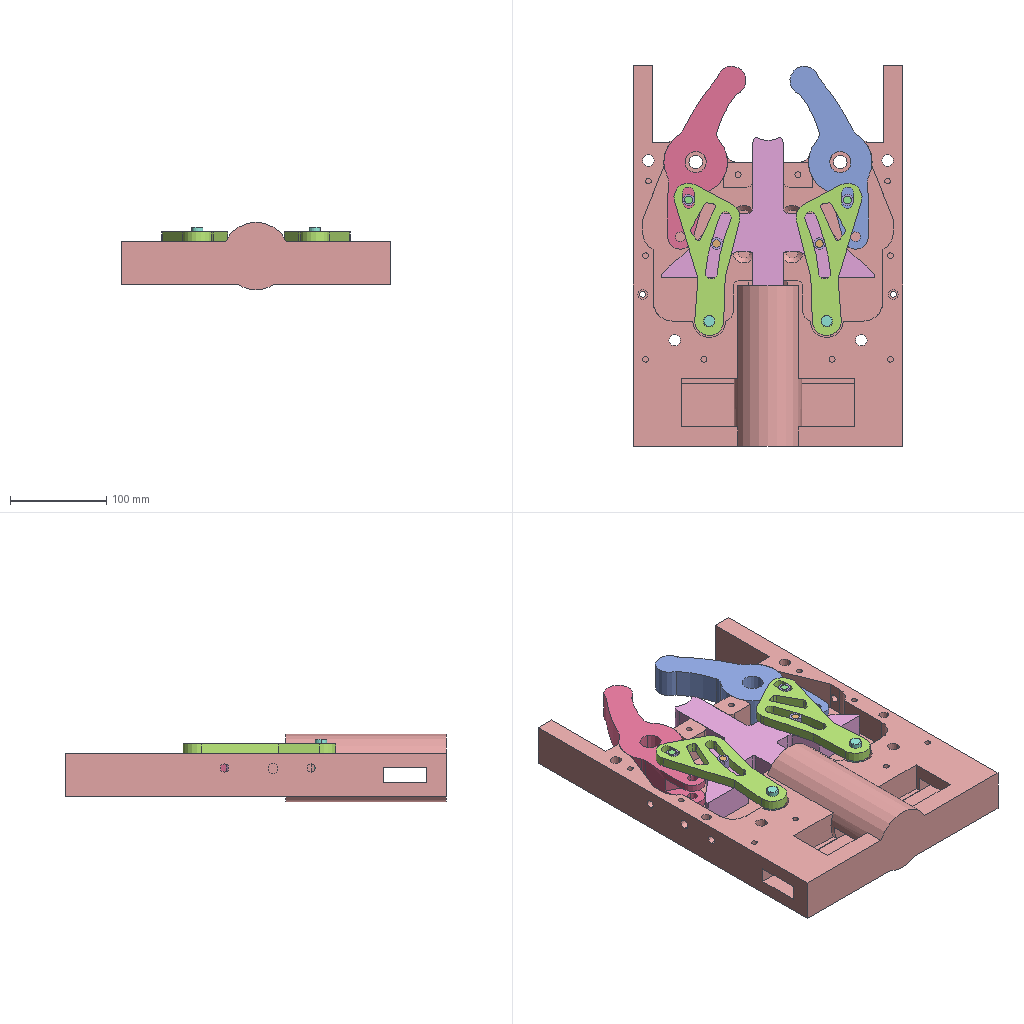Assembly | SolidWorks | 10 different items | 17 placed | box 280 x 395 x 70 mm
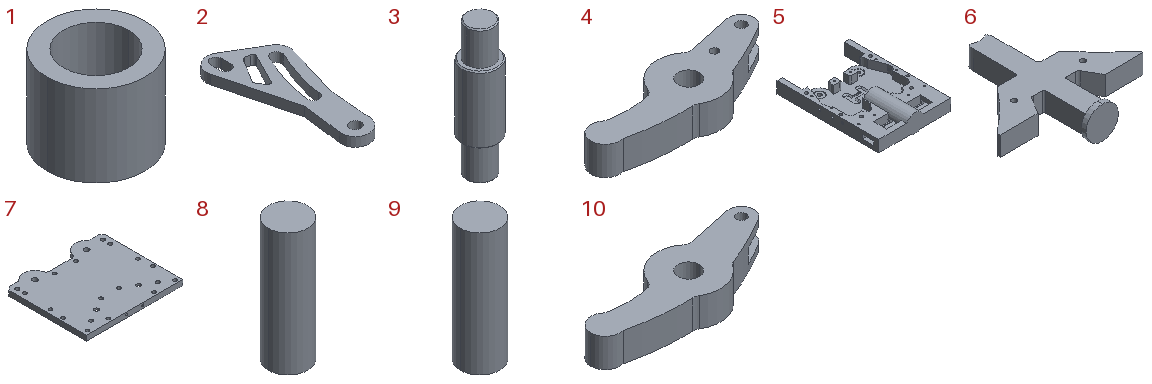Parts list (item | quantity | size | volume | features):
1 | x4 | 12 x 12 x 10 mm | 628.319 mm3 | features Extrusion 1
2 | x2 | 67.492 x 158.964 x 10 mm | 45368 mm3 | features Cut 2, ICE 2, Extrusion 1
3 | x2 | 16 x 16 x 60 mm | 9403 mm3 | features ICE 2, Chamfer 1, Extrusion 1
4 | x1 | 196.199 x 67.267 x 30 mm | 199091 mm3 | features ICE 15, Cut 1, Extrusion 1, Fillet 1
5 | x1 | 280 x 394.673 x 70 mm | 2510782 mm3 | features Attribute 187, ICE 26, Cut 11, Chamfer 4, Fillet 3, Extrusion 1, MirrorPattern 1
6 | x1 | 221.447 x 193.66 x 50 mm | 400373 mm3 | features ICE 17, Cut 4, Chamfer 2, Extrusion 1, Fillet 1, MirrorPattern 1
7 | x1 | 280 x 247.673 x 15 mm | 750844 mm3 | features Cut 14, ICE 14, Fillet 2, Chamfer 1, Extrusion 1
8 | x2 | 8 x 8 x 25 mm | 1257 mm3 | features Extrusion 1
9 | x2 | 8 x 8 x 25 mm | 1257 mm3 | features Extrusion 1
10 | x1 | 196.199 x 67.267 x 30 mm | 199091 mm3 | features ICE 15, Cut 1, Extrusion 1, Fillet 1
Mates (type | each side: item.copy, entity, surface, feature):
Concentric | 5.1 face cylinder Cut-Extrude2 | 10.1 face cylinder Cut-Extrude13
Coincident | 5.1 face plane Boss-Extrude1 | 10.1 face plane Boss-Extrude3
Concentric | 5.1 face cylinder Cut-Extrude7 | 2.1 face cylinder Cut-Extrude14
Coincident | 5.1 face plane Boss-Extrude1 | 6.1 face plane Boss-Extrude3
Concentric | 5.1 face cylinder Cut-Extrude7 | 3.1 face cylinder Boss-Extrude3
Coincident | 5.1 face plane Boss-Extrude1 | 3.1 face plane Boss-Extrude2
Concentric | 6.1 face cylinder Cut-Extrude14 | 8.1 face cylinder Boss-Extrude1
Coincident | 6.1 face plane Cut-Extrude14 | 8.1 face plane Boss-Extrude1
Concentric | 8.1 face cylinder Boss-Extrude1 | 1.1 face cylinder Boss-Extrude1
Coincident | 6.1 face plane Boss-Extrude1 | 1.1 face plane Boss-Extrude1
Concentric | 9.1 face cylinder Boss-Extrude1 | 1.2 face cylinder Boss-Extrude1
Concentric | 3.1 face cylinder Boss-Extrude1 | 2.2 face cylinder Cut-Extrude14
Concentric | 5.1 face cylinder Cut-Extrude2 | 4.1 face cylinder Cut-Extrude13
Coincident | 5.1 face plane Boss-Extrude1 | 4.1 face plane Boss-Extrude5
Concentric | 9.1 face cylinder Boss-Extrude1 | 4.1 face cylinder Cut-Extrude17
Coincident | 1.2 face plane Boss-Extrude1 | 4.1 face plane Boss-Extrude3
Concentric | 5.1 face cylinder Cut-Extrude7 | 3.2 face cylinder Boss-Extrude3
Coincident | 5.1 face plane Boss-Extrude1 | 3.2 face plane Boss-Extrude2
Concentric | 6.1 face cylinder Cut-Extrude15 | 8.2 face cylinder Boss-Extrude1
Coincident | 6.1 face plane Cut-Extrude15 | 8.2 face plane Boss-Extrude1
Concentric | 1.3 face cylinder Boss-Extrude1 | 8.2 face cylinder Boss-Extrude1
Coincident | 6.1 face plane Boss-Extrude1 | 1.3 face plane Boss-Extrude1
Concentric | 9.2 face cylinder Boss-Extrude1 | 1.4 face cylinder Boss-Extrude1
Concentric | 10.1 face cylinder Cut-Extrude18 | 9.2 face cylinder Boss-Extrude1
Coincident | 10.1 face plane Cut-Extrude18 | 9.2 face plane Boss-Extrude1
Coincident | 10.1 face plane Boss-Extrude5 | 1.4 face plane Boss-Extrude1
Tangent | 2.1 face surface:4009 Cut-Extrude15 | 1.3 face cylinder Boss-Extrude1
Tangent | 2.1 face plane Cut-Extrude8 | 1.4 face cylinder Boss-Extrude1
Coincident | 6.1 face plane Boss-Extrude1 | 2.2 face plane Boss-Extrude1
Tangent | 1.1 face cylinder Boss-Extrude1 | 2.2 face surface:4009 Cut-Extrude15
Tangent | 1.2 face cylinder Boss-Extrude1 | 2.2 face plane Cut-Extrude8
Coincident | 5.1 face plane Boss-Extrude3 | 6.1 face plane Boss-Extrude6